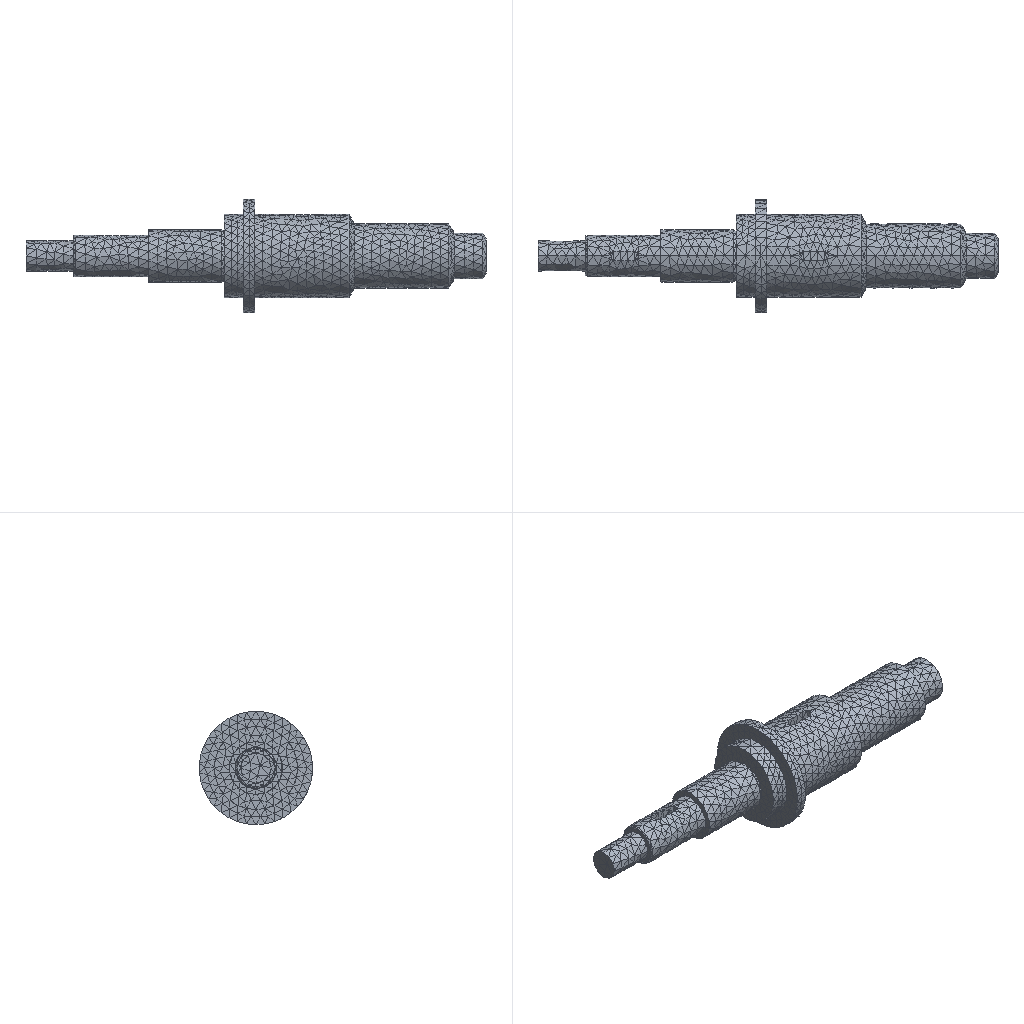Simulation study | ansys workbench
Set-up summary:
category,name,step,type,value,unit,region
solver,ansys_mapdl
solver,version,,,24.2
units,MPA,,stated
analysis,deck,,static,static
load_step,requested,,,1
analysis,nlgeom,,,False
mesh,nodes,,,23898
mesh,elements,,,16031
element_type,ANSYS 187 (type 1),,solid,15559
element_type,ANSYS 174 (type 2),,contact,472
element_type,ANSYS 170 (type 3),,target,0
load,load commands in deck,,count,3
bc,support commands in deck,,count,1
named_set,_FIXEDSU,,component
material,1,,in results
check,setup vs results,,match,results also hold 0 node(s) and 1 element(s) the deck makes with ['EN']; those were not compared; 1 node(s) the solver created internally for pilot nodes (ZST-1/廷旭-23个(1)/有限元仿真/扭转/扭转_files/dp0/SYS/MECH/solve.out) are in the results only
Ansys APDL input file, long lists of numbers shortened:
/batch
/config,noeldb,1     ! force off writing results to database
*get,_wallstrt,active,,time,wall
! ANSYS input file written by Workbench version 2024 R2
! File used for geometry attach: C:\Users\USER_\Desktop\zhou.STEP
/title,wbnew--____ (A5)
! ****** Begin Custom Load Command Snippet ******
/COM, ACT Extensions:
/COM,     LSDYNA, 2024.2
/COM,/COM,     ANSYSMotion, 2024.2
/COM,
! ****** End   Custom Load Command Snippet ******
*DIM,_wb_ProjectScratch_dir,string,248
_wb_ProjectScratch_dir(1) = 'C:\Users\USER_\AppData\Local\Temp\WB_86130_263296_6\_ProjectScratch\ScrD3C3\'
*DIM,_wb_SolverFiles_dir,string,248
_wb_SolverFiles_dir(1) = 'C:\Users\USER_\AppData\Local\Temp\WB_86130_263296_6\wbnew_files\dp0\SYS\MECH\'
*DIM,_wb_userfiles_dir,string,248
_wb_userfiles_dir(1) = 'C:\Users\USER_\AppData\Local\Temp\WB_86130_263296_6\wbnew_files\user_files\'
/com,--- Data in consistent NMM units. See Solving Units in the help system for more information.
/units,MPA
/nopr
/wb,file,start              !  signify a WB generated input file
/prep7
! Turn off shape checking because checks already performed inside WB mesher.
! See help system for more information.
SHPP,OFF,,NOWARN
/nolist
etcon,set             ! allow ANSYS to choose best KEYOP's for 180x elements, resets any applicable keyopt to MAPDL defaults
/com,*********** Nodes for the whole assembly ***********
nblock,3,,26286
(1i9,3e20.9e3)
        1    -1.983603948E+01     2.500000000E+00     2.185749299E+01
! (23896 more lines like these left out)
-1
/com,*********** Nodes for all Remote Points ***********
nblock,3
(1i9,3e20.9e3)
    23898     3.855071211E+01    -8.881784197E-16    -3.415641928E-16
-1
/wb,elem,start            !  set before creation of elements
/com,*********** Elements for Body 1 'zhou-FreeParts|____-____2' ***********
et,1,187
eblock,19,solid,,15559
(19i9)
        1        1        1        1        0        0        0        0       10        0        1      161     3421     1225     3406     4681    11717     4677     4680
! (31117 more lines like these left out)
-1
/wb,elem,end               !  done creating elements
/com,*********** Send User Defined Coordinate System(s) ***********
csys,0
toffst,273.15,      ! Temperature offset from absolute zero
/com,*********** Set Reference Temperature ***********
tref,22.
/wb,mat,start              !  starting to send materials
/com,*********** Send Materials ***********
Temperature = 'TEMP' ! Temperature
MP,DENS,1,7.85e-09,	! tonne mm^-3
MP,ALPX,1,1.2e-05,	! C^-1
MP,C,1,434000000,	! mm^2 s^-2 C^-1
MP,KXX,1,60.5,	! tonne mm s^-3 C^-1
MP,RSVX,1,0.00017,	! ohm mm
MP,EX,1,200000,	! tonne s^-2 mm^-1
MP,NUXY,1,0.3,
MP,MURX,1,10000,
/wb,mat,end                !  done sending materials
!************************* Model Summary ********************
!zhou-FreeParts|____-____2,	ç»æé¢,	matid,	1
!************************* End Model Summary ********************
! get the diagonal of the bounding box. Needed later for other things
*get,_xmin,node,,mnloc,x
*get,_ymin,node,,mnloc,y
*get,_zmin,node,,mnloc,z
*get,_xmax,node,,mxloc,x
*get,_ymax,node,,mxloc,y
*get,_zmax,node,,mxloc,z
_ASMDIAG=(_xmax-_xmin)*(_xmax-_xmin)+(_ymax-_ymin)*(_ymax-_ymin)+(_zmax-_zmin)*(_zmax-_zmin)
_ASMDIAG=SQRT(_ASMDIAG)
/wb,contact,start          !  starting to send contact
/wb,contact,end            !  done creating contacts
/golist
/wb,load,start             !  starting to send loads
/com,*********** Fixed Supports ***********
CMBLOCK,_FIXEDSU,NODE,       49
(8i10)
        78        83        84        85        86        87        88       493
       494       495       496       497      1490      1491      1492      1493
      4002      4003      4004      4042      4044      4045      4046      4048
      4051      4053      4056      4059      4062      4063      4065      4068
      4072      4073      7315      7317      7319      7322      7323      7325
      7328      7331      7334      7337     13097     13098     13099     13104
     13105
cmsel,s,_FIXEDSU
d,all,all
nsel,all
/com,*********** Create Remote Point "ÄÚ²¿Ô¶³Ìµã" ***********
! -------- Remote Point Used by "Á¦¾Ø" --------
*set,tid,3
*set,cid,2
et,cid,174
et,tid,170
keyo,tid,2,1               ! Don't fix the pilot node
keyo,tid,4,111111
keyo,cid,12,5              ! Bonded Contact
keyo,cid,4,1               ! Deformable RBE3 style load
keyo,cid,2,2               ! MPC style contact
eblock,10,,,472
(15i9)
    18555        2        2        2        0      454      136      145      145     4422     4419      145     4503
! (471 more lines like these left out)
-1
*set,_npilot,23898
_npilot35=_npilot
type,tid
mat ,cid
real,cid
tshape,pilo
en,19027,_npilot
tshape
/com,*********** Construct Moment Using Remote Attachment ***********
/gst,on,on
fini
*get,_numnode,node,0,count
*get,_numelem,elem,0,count
*get, _MAXELEMNUM, elem, 0, NUM, MAX
*get, _MAXNODENUM, node, 0, NUM, MAX
*get, _MAXELEMTYPE, etyp, 0, NUM, MAX
*get, _MAXREALCONST, rcon, 0, NUM, MAX
/go
/wb,load,end               !  done creating loads
/com,--- Number of total nodes = %_numnode%
/com,--- Number of contact elements = 472
/com,--- Number of spring elements = 0
/com,--- Number of bearing elements = 0
/com,--- Number of solid elements = 15559
/com,--- Number of condensed parts = 0
/com,--- Number of total elements = %_numelem%
*get,_wallbsol,active,,time,wall
/com,****************************************************************************
/com,*************************    SOLUTION       ********************************
/com,****************************************************************************
/solu
antype,0                   ! static analysis
_thickRatio=  1     ! Ratio of thick parts in the model
eqsl,pcg,1e-8,,,,,,1
cntr,print,1               ! print out contact info and also make no initial contact an error
cncheck,dmp		!	Enable program controlled contact splitting for distributed memory parallel run
dmpoption,emat,no             ! Don't combine emat file for DANSYS
dmpoption,esav,no             ! Don't combine esav file for DANSYS
nldiag,cont,iter           ! print out contact info each equilibrium iteration
rescontrol,,none                 ! Do not keep any restart files
/com,****************************************************
/com,******************* SOLVE FOR LS 1 OF 1 ****************
nsel,s,node,,23898
f,all,mx,20000.
f,all,my,0.
f,all,mz,0.
nsel,all
/nopr
/gopr
nsub,1,1,1
time,1.
outres,erase
outres,all,none
outres,nsol,all,
outres,rsol,all
outres,eangl,all
outres,etmp,all
outres,veng,all
outres,strs,all,
outres,epel,all,
outres,eppl,all,
outres,cont,all,
! *********** WB SOLVE COMMAND ***********
! check interactive state
*get,ANSINTER_,active,,int
*if,ANSINTER_,ne,0,then
/eof
*endif
solve
/com *************** Write FE CONNECTORS *********
CEWRITE,file,ce,,INTE
/com,****************************************************
/com,*************** FINISHED SOLVE FOR LS 1 *************
*get,_wallasol,active,,time,wall
/nopr
*get,_numnode,node,0,count
*get,_numelem,elem,0,count
*get, _MAXELEMNUM, elem, 0, NUM, MAX
*get, _MAXNODENUM, node, 0, NUM, MAX,,,INTERNAL
*get, _MAXELEMTYPE, etyp, 0, NUM, MAX
*get, _MAXREALCONST, rcon, 0, NUM, MAX
*get,_NSOLTHREADS,active,0,ntfs
*get,_NSOLPROCESSES,active,0,npfs
/gopr
*get,_PCGITER,active,,solu,cgiter
/post1
xmlo,ENCODING,ISO-8859-1
xmlo,parm
/xml,parm,xml
fini
/gopr
*get,_walldone,active,,time,wall
_preptime=(_wallbsol-_wallstrt)*3600
_solvtime=(_wallasol-_wallbsol)*3600
_posttime=(_walldone-_wallasol)*3600
_totaltim=(_walldone-_wallstrt)*3600
*get,_dlbratio,active,0,solu,dlbr
*get,_combtime,active,0,solu,comb
*get,_ssmode,active,0,solu,ssmm
*get,_ndofs,active,0,solu,ndof
*get,_sol_end_time,active,0,set,time
*if,_sol_end_time,eq,1.,then
/fclean				!clean distributed files
*endif
/com,--- Total number of nodes = %_numnode%
/com,--- Total number of elements = %_numelem%
/com,--- Element load balance ratio = %_dlbratio%
/com,--- Time to combine distributed files = %_combtime%
/com,--- Sparse memory mode = %_ssmode%
/com,--- Number of DOF = %_ndofs%
/wb,file,end               ! done with WB generated input
Results summary:
result,analysis,,,static
result,last_loadstep,,,1
result,primary field,,,displacement
result,reaction total,1,FX,-3e-06,N
result,reaction total,1,FY,3e-06,N
result,reaction total,1,FZ,-2e-06,N
result,mass,,,0.001647,"NMM: mm, ton, N, s, mV, mA, degC"